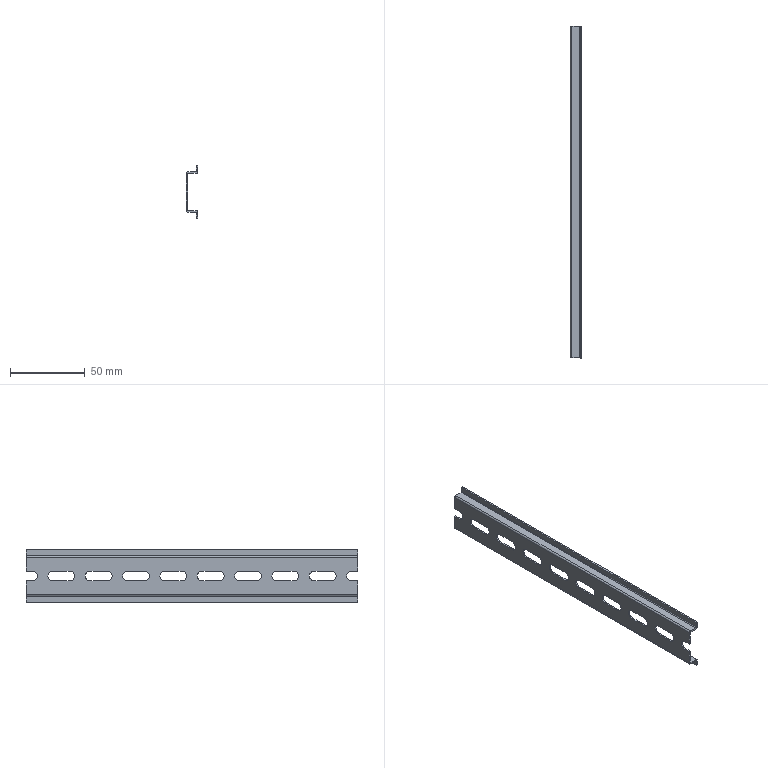Part | SolidWorks | features BaseBody 1 | 1 solid | 71 faces | box 7.5 x 222.25 x 35 mm | volume 9598 mm3 | plane 36 | cylinder 35 | commonest cylinder face diameters 6.3 x27 1 x4 2 x4